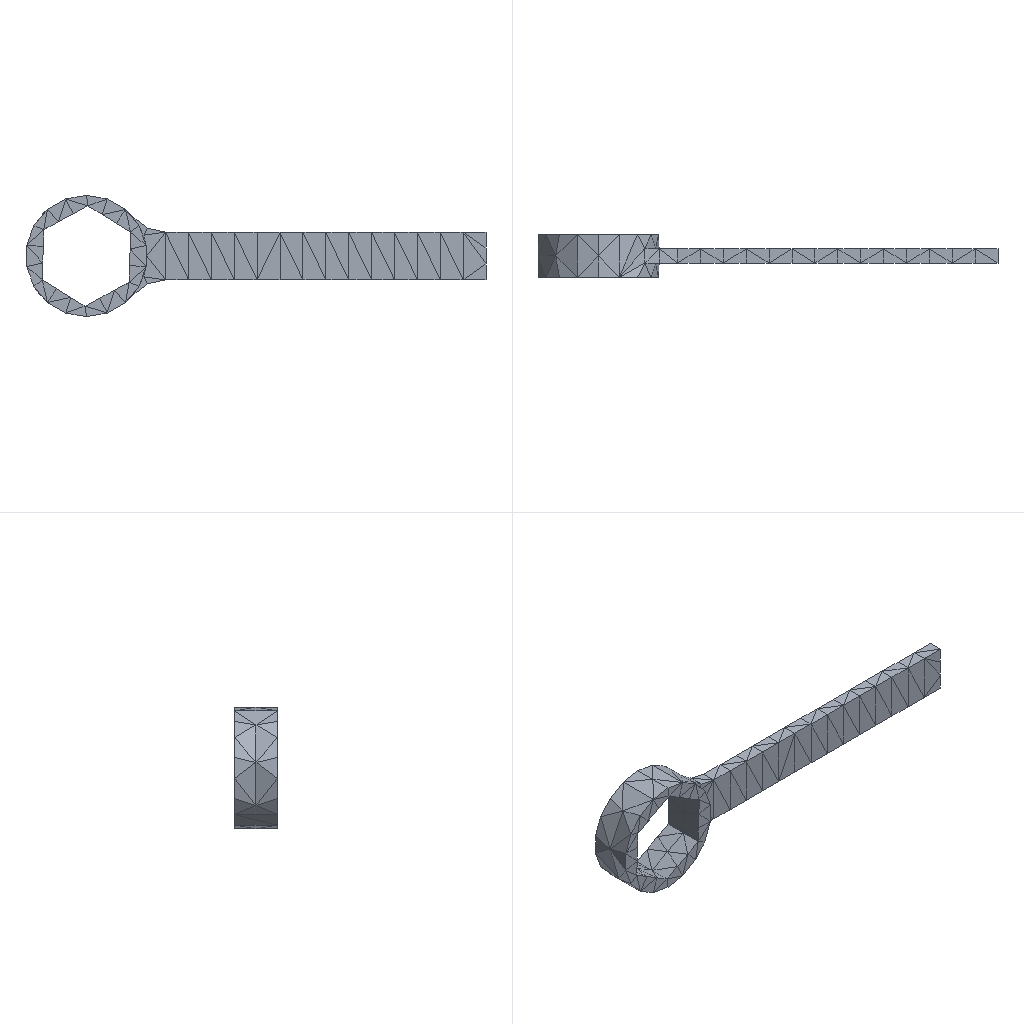Simulation study | ansys workbench
Set-up summary:
category,name,step,type,value,unit,region
solver,ansys_workbench
units,mm-N-s-tonne (MPa),,stated,"/units,MPA"
analysis,LS1,,static
load_step,LS1,LS1,static,nsubst=1; time=1
mesh,nodes,,,810
mesh,elements,,,335
element_type,SOLID187,,,307
element_type,SURF154,,,28
material,Structural Steel,,E,200000,tonne s^-2 mm^-1
material,Structural Steel,,nu,0.3
material,Structural Steel,,density,7.85e-09,tonne mm^-3
material,Structural Steel,,conductivity,60.5,tonne mm s^-3 C^-1
material,Structural Steel,,specific_heat,4.34e+08,mm^2 s^-2 C^-1
material,Structural Steel,,cte,1.2e-05,C^-1
material,Structural Steel,,permeability,10000
material,Structural Steel,,resistivity,0.00017,ohm mm
load,Define Force Using Surface Effect Elements,LS1,surface-effect pres face 1,6.14127e-19,,SURF154 #2
load,Define Force Using Surface Effect Elements,LS1,surface-effect pres face 3,-0.02135,,SURF154 #2
bc,Fixed Supports,model,fixed,[dofs=ALL],,_FIXEDSU
named_set,_FIXEDSU,,node,156
Ansys APDL input file, long lists of numbers shortened:
/batch
/config,noeldb,1     ! force off writing results to database
*get,_wallstrt,active,,time,wall
! ANSYS input file written by Workbench version 2022 R1
! File used for geometry attach:
/title,wbnew--____ (A5)
! ****** Begin Custom Load Command Snippet ******
/COM, ACT Extensions:
/COM,     LSDYNA, 2021.1
/COM,
! ****** End   Custom Load Command Snippet ******
*DIM,_wb_ProjectScratch_dir,string,248
_wb_ProjectScratch_dir(1) = ''
*DIM,_wb_SolverFiles_dir,string,248
_wb_SolverFiles_dir(1) = ''
*DIM,_wb_userfiles_dir,string,248
_wb_userfiles_dir(1) = ''
/com,--- Data in consistent NMM units. See Solving Units in the help system for more information.
/units,MPA
/nopr
/wb,file,start              !  signify a WB generated input file
/prep7
! Turn off shape checking because checks already performed inside WB mesher.
! See help system for more information.
SHPP,OFF,,NOWARN
/nolist
etcon,set             ! allow ANSYS to choose best KEYOP's for 180x elements, resets any applicable keyopt to MAPDL defaults
/com,*********** Nodes for the whole assembly ***********
nblock,3,,891
(1i9,3e20.9e3)
        1     5.215332488E-15     2.000000000E+01     4.258642159E+01
! (809 more lines like these left out)
-1
/wb,elem,start            !  set before creation of elements
/com,*********** Elements for Body 1 "__-FreeParts|__-__3" ***********
et,1,187
eblock,19,solid,,307
(19i9)
        1        1        1        1        0        0        0        0       10        0        1       24      136      164       28      297      746      299      294
! (613 more lines like these left out)
-1
/wb,elem,end               !  done creating elements
/com,*********** Send User Defined Coordinate System(s) ***********
csys,0
toffst,273.15,  ! Temperature offset from absolute zero
/com,*********** Set Reference Temperature ***********
tref,22.
/wb,mat,start              !  starting to send materials
/com,*********** Send Materials ***********
Temperature = 'TEMP' ! Temperature
MP,DENS,1,7.85e-09,	! tonne mm^-3
MP,ALPX,1,1.2e-05,	! C^-1
MP,C,1,434000000,	! mm^2 s^-2 C^-1
MP,KXX,1,60.5,	! tonne mm s^-3 C^-1
MP,RSVX,1,0.00017,	! ohm mm
MP,EX,1,200000,	! tonne s^-2 mm^-1
MP,NUXY,1,0.3,
MP,MURX,1,10000,
/wb,mat,end                !  done sending materials
!************************* Model Summary ********************
!__-FreeParts|__-__3,	结构钢,	matid,	1
!************************* End Model Summary ********************
! get the diagonal of the bounding box. Needed later for other things
*get,_xmin,node,,mnloc,x
*get,_ymin,node,,mnloc,y
*get,_zmin,node,,mnloc,z
*get,_xmax,node,,mxloc,x
*get,_ymax,node,,mxloc,y
*get,_zmax,node,,mxloc,z
_ASMDIAG=(_xmax-_xmin)*(_xmax-_xmin)+(_ymax-_ymin)*(_ymax-_ymin)+(_zmax-_zmin)*(_zmax-_zmin)
_ASMDIAG=SQRT(_ASMDIAG)
/wb,contact,start          !  starting to send contact
/wb,contact,end            !  done creating contacts
/golist
/wb,load,start             !  starting to send loads
/com,*********** Fixed Supports ***********
CMBLOCK,_FIXEDSU,NODE,      156
(8i10)
       117       118       119       120       121       122       123       124
! (19 more lines like these left out)
cmsel,s,_FIXEDSU
d,all,all
nsel,all
/com,*********** Define Force Using Surface Effect Elements ***********
local,12,0,0.,0.,0.,0.,0.,0.
csys,0
et,2,154
eblock,10,,,28
(15i9)
      642        2        2        2       12       54       70       53       53      484      482       53      481
! (27 more lines like these left out)
-1
esel,s,type,,2
keyop,2,2,1                ! Apply load in local coordinate system
keyop,2,7,1                ! Use original area so load is constant in large deformation
esel,all
/gst,on,on
fini
*get,_numnode,node,0,count
*get,_numelem,elem,0,count
*get, _MAXELEMNUM, elem, 0, NUM, MAX
*get, _MAXNODENUM, node, 0, NUM, MAX
*get, _MAXELEMTYPE, etyp, 0, NUM, MAX
*get, _MAXREALCONST, real, 0, NUM, MAX
/go
/wb,load,end               !  done creating loads
/com,--- Number of total nodes = %_numnode%
/com,--- Number of contact elements = 28
/com,--- Number of spring elements = 0
/com,--- Number of bearing elements = 0
/com,--- Number of solid elements = 307
/com,--- Number of condensed parts = 0
/com,--- Number of total elements = %_numelem%
*get,_wallbsol,active,,time,wall
/com,****************************************************************************
/com,*************************    SOLUTION       ********************************
/com,****************************************************************************
/solu
antype,0                   ! static analysis
_thickRatio=  0     ! Ratio of thick parts in the model
eqsl,sparse,,,,,1
cntr,print,1               ! print out contact info and also make no initial contact an error
dmpoption,emat,no             ! Don't combine emat file for DANSYS
dmpoption,esav,no             ! Don't combine esav file for DANSYS
nldiag,cont,iter           ! print out contact info each equilibrium iteration
rescontrol,,none                 ! Do not keep any restart files
/com,****************************************************
/com,******************* SOLVE FOR LS 1 OF 1 ****************
esel,s,type,,2
nsle
sfe,all,1,pres,1,6.14127063563927e-019
sfe,all,2,pres,1,0.
sfe,all,3,pres,1,-2.13487999116454e-002
nsel,all
esel,all
/nopr
/gopr
nsub,1,1,1
time,1.
outres,erase
outres,all,none
outres,nsol,all,
outres,rsol,all
outres,eangl,all
outres,etmp,all
outres,veng,all
outres,strs,all,
outres,epel,all,
outres,eppl,all,
outres,cont,all,
! *********** WB SOLVE COMMAND ***********
! check interactive state
*get,ANSINTER_,active,,int
*if,ANSINTER_,ne,0,then
/eof
*endif
solve
/com *************** Write FE CONNECTORS *********
CEWRITE,file,ce,,INTE
/com,****************************************************
/com,*************** FINISHED SOLVE FOR LS 1 *************
*get,_wallasol,active,,time,wall
/nopr
*get,_numnode,node,0,count
*get,_numelem,elem,0,count
*get, _MAXELEMNUM, elem, 0, NUM, MAX
*get, _MAXNODENUM, node, 0, NUM, MAX,,,INTERNAL
*get, _MAXELEMTYPE, etyp, 0, NUM, MAX
*get, _MAXREALCONST, real, 0, NUM, MAX
/gopr
/post1
xmlo,ENCODING,ISO-8859-1
xmlo,parm
/xml,parm,xml
fini
/gopr
*get,_walldone,active,,time,wall
_preptime=(_wallbsol-_wallstrt)*3600
_solvtime=(_wallasol-_wallbsol)*3600
_posttime=(_walldone-_wallasol)*3600
_totaltim=(_walldone-_wallstrt)*3600
*get,_dlbratio,active,0,solu,dlbr
*get,_combtime,active,0,solu,comb
*get,_ssmode,active,0,solu,ssmm
*get,_ndofs,active,0,solu,ndof
*get,_sol_end_time,active,0,set,time
*if,_sol_end_time,eq,1.,then
/fclean				!clean distributed files
*endif
/com,--- Total number of nodes = %_numnode%
/com,--- Total number of elements = %_numelem%
/com,--- Element load balance ratio = %_dlbratio%
/com,--- Time to combine distributed files = %_combtime%
/com,--- Sparse memory mode = %_ssmode%
/com,--- Number of DOF = %_ndofs%
/wb,file,end               ! done with WB generated input
Results summary:
result,analyses[0].index,,,1
result,analyses[0].system,,,SYS
result,analyses[0].deck,,,deck.dat
result,analyses[0].solve_status,,,completed
result,analyses[0].analysis_type,,,static
result,analyses[0].physics,,,mechanical
result,analyses[0].unit_system,,,"NMM: mm, ton, N, s, mV, mA, degC"
result,analyses[0].n_sets,,,1
result,analyses[0].load_steps[0].set,set=1,,1
result,analyses[0].load_steps[0].time_or_freq,set=1,,1
result,analyses[0].load_steps[0].max_displacement_magnitude,set=1,,0.0145
result,analyses[0].load_steps[0].max_von_mises_nodal,set=1,,3.065
result,analyses[0].load_steps[0].reaction_force_sum_xyz[1],set=1,,-1.59876e-08
result,analyses[0].load_steps[0].reaction_force_sum_xyz[2],set=1,,1.69489e-08
result,analyses[0].load_steps[0].reaction_force_sum_xyz[3],set=1,,48